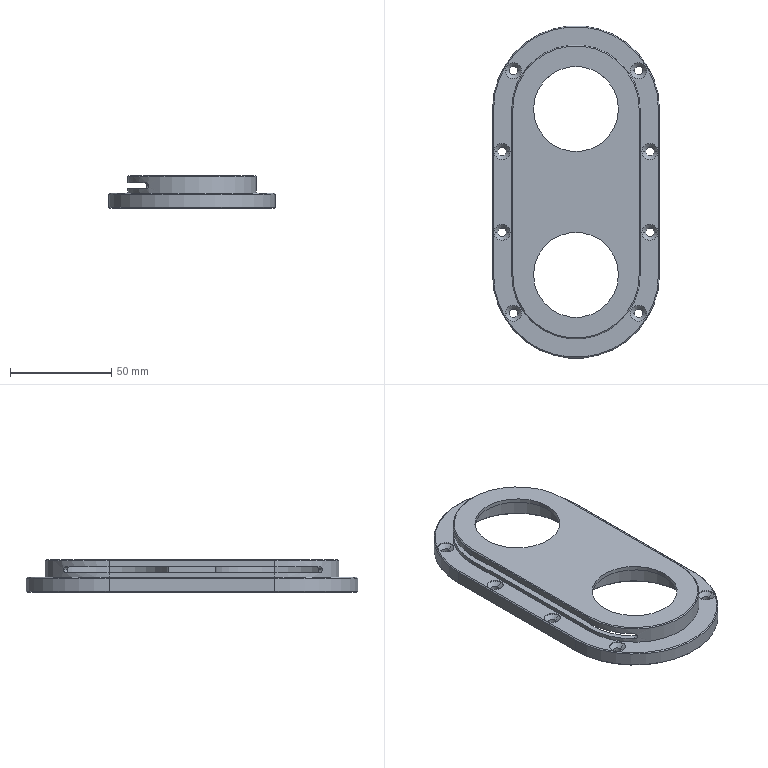Part | SolidWorks | features ICE 5, Chamfer 2, HoleWzd 2, Cut 1, Extrusion 1, Fillet 1, MoveFace 1 | 1 solid | 101 faces | box 82.5 x 164.5 x 16 mm | volume 70978 mm3 | cylinder 52 | cone 30 | plane 19 | commonest cylinder face diameters 4.2 x16 8 x16 3 x4 42 x4 58.5 x4 61.5 x4